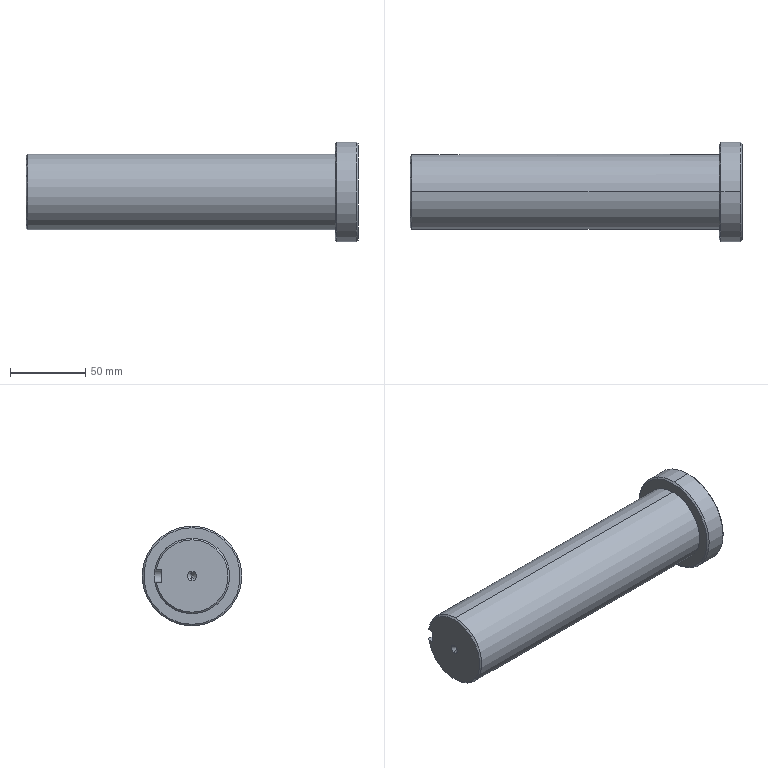Part | SolidWorks | features BaseBody 1 | 1 solid | 22 faces | box 220 x 66 x 66 mm | volume 452201 mm3 | cone 11 | plane 6 | cylinder 5 | commonest cylinder face diameters 50 x2 66 x2 8 x1
STEP:
#1=CARTESIAN_POINT('',(-110.,0.,24.));
#2=VERTEX_POINT('',#1);
#3=CARTESIAN_POINT('',(-110.,23.664,4.));
#4=VERTEX_POINT('',#3);
#5=CARTESIAN_POINT('',(-110.,0.,0.));
#6=DIRECTION('',(-1.,0.,0.));
#7=DIRECTION('',(0.,0.,-1.));
#8=AXIS2_PLACEMENT_3D('',#5,#6,#7);
#9=CIRCLE('',#8,24.);
#10=EDGE_CURVE('',#2,#4,#9,.T.);
#11=ORIENTED_EDGE('',*,*,#10,.F.);
#12=CARTESIAN_POINT('',(-109.,0.,25.));
#13=VERTEX_POINT('',#12);
#14=CARTESIAN_POINT('',(-110.,0.,24.));
#15=DIRECTION('',(0.7071,0.,0.7071));
#16=VECTOR('',#15,1000.);
#17=LINE('',#14,#16);
#18=EDGE_CURVE('',#2,#13,#17,.T.);
#19=ORIENTED_EDGE('',*,*,#18,.T.);
#20=CARTESIAN_POINT('',(-109.,24.678,4.));
#21=VERTEX_POINT('',#20);
#22=CARTESIAN_POINT('',(-109.,0.,0.));
#23=DIRECTION('',(1.,0.,0.));
#24=DIRECTION('',(0.,0.,-1.));
#25=AXIS2_PLACEMENT_3D('',#22,#23,#24);
#26=CIRCLE('',#25,25.);
#27=EDGE_CURVE('',#21,#13,#26,.T.);
#28=ORIENTED_EDGE('',*,*,#27,.F.);
#29=CARTESIAN_POINT('',(-110.,23.664,4.));
#30=CARTESIAN_POINT('',(-109.667,24.002,4.));
#31=CARTESIAN_POINT('',(-109.333,24.34,4.));
#32=CARTESIAN_POINT('',(-109.,24.678,4.));
#33=B_SPLINE_CURVE_WITH_KNOTS('',3,(#29,#30,#31,#32),.UNSPECIFIED.,.F.,.F.,(4,4),(0.007277,0.008701),.UNSPECIFIED.);
#34=EDGE_CURVE('',#4,#21,#33,.T.);
#35=ORIENTED_EDGE('',*,*,#34,.F.);
#36=EDGE_LOOP('',(#11,#19,#28,#35));
#37=FACE_OUTER_BOUND('',#36,.T.);
#38=CARTESIAN_POINT('',(-110.,0.,0.));
#39=DIRECTION('',(1.,0.,0.));
#40=DIRECTION('',(0.,0.,-1.));
#41=AXIS2_PLACEMENT_3D('',#38,#39,#40);
#42=CONICAL_SURFACE('',#41,24.,0.7854);
#43=ADVANCED_FACE('',(#37),#42,.T.);
#44=ORIENTED_EDGE('',*,*,#18,.F.);
#45=CARTESIAN_POINT('',(-110.,0.,-24.));
#46=VERTEX_POINT('',#45);
#47=CARTESIAN_POINT('',(-110.,0.,0.));
#48=DIRECTION('',(-1.,0.,0.));
#49=DIRECTION('',(0.,0.,-1.));
#50=AXIS2_PLACEMENT_3D('',#47,#48,#49);
#51=CIRCLE('',#50,24.);
#52=EDGE_CURVE('',#46,#2,#51,.T.);
#53=ORIENTED_EDGE('',*,*,#52,.F.);
#54=CARTESIAN_POINT('',(-109.,0.,-25.));
#55=VERTEX_POINT('',#54);
#56=CARTESIAN_POINT('',(-110.,0.,-24.));
#57=DIRECTION('',(0.7071,0.,-0.7071));
#58=VECTOR('',#57,1000.);
#59=LINE('',#56,#58);
#60=EDGE_CURVE('',#46,#55,#59,.T.);
#61=ORIENTED_EDGE('',*,*,#60,.T.);
#62=CARTESIAN_POINT('',(-109.,0.,0.));
#63=DIRECTION('',(1.,0.,0.));
#64=DIRECTION('',(0.,0.,-1.));
#65=AXIS2_PLACEMENT_3D('',#62,#63,#64);
#66=CIRCLE('',#65,25.);
#67=EDGE_CURVE('',#13,#55,#66,.T.);
#68=ORIENTED_EDGE('',*,*,#67,.F.);
#69=EDGE_LOOP('',(#44,#53,#61,#68));
#70=FACE_OUTER_BOUND('',#69,.T.);
#71=CARTESIAN_POINT('',(-110.,0.,0.));
#72=DIRECTION('',(1.,0.,0.));
#73=DIRECTION('',(0.,0.,-1.));
#74=AXIS2_PLACEMENT_3D('',#71,#72,#73);
#75=CONICAL_SURFACE('',#74,24.,0.7854);
#76=ADVANCED_FACE('',(#70),#75,.T.);
#77=CARTESIAN_POINT('',(95.,0.,32.));
#78=VERTEX_POINT('',#77);
#79=CARTESIAN_POINT('',(95.,0.,-32.));
#80=VERTEX_POINT('',#79);
#81=CARTESIAN_POINT('',(95.,0.,0.));
#82=DIRECTION('',(-1.,0.,0.));
#83=DIRECTION('',(0.,0.,-1.));
#84=AXIS2_PLACEMENT_3D('',#81,#82,#83);
#85=CIRCLE('',#84,32.);
#86=EDGE_CURVE('',#78,#80,#85,.T.);
#87=ORIENTED_EDGE('',*,*,#86,.F.);
#88=CARTESIAN_POINT('',(96.,0.,33.));
#89=VERTEX_POINT('',#88);
#90=CARTESIAN_POINT('',(95.,0.,32.));
#91=DIRECTION('',(0.7071,0.,0.7071));
#92=VECTOR('',#91,1000.);
#93=LINE('',#90,#92);
#94=EDGE_CURVE('',#78,#89,#93,.T.);
#95=ORIENTED_EDGE('',*,*,#94,.T.);
#96=CARTESIAN_POINT('',(96.,0.,-33.));
#97=VERTEX_POINT('',#96);
#98=CARTESIAN_POINT('',(96.,0.,0.));
#99=DIRECTION('',(1.,0.,0.));
#100=DIRECTION('',(0.,0.,-1.));
#101=AXIS2_PLACEMENT_3D('',#98,#99,#100);
#102=CIRCLE('',#101,33.);
#103=EDGE_CURVE('',#97,#89,#102,.T.);
#104=ORIENTED_EDGE('',*,*,#103,.F.);
#105=CARTESIAN_POINT('',(95.,0.,-32.));
#106=DIRECTION('',(0.7071,0.,-0.7071));
#107=VECTOR('',#106,1000.);
#108=LINE('',#105,#107);
#109=EDGE_CURVE('',#80,#97,#108,.T.);
#110=ORIENTED_EDGE('',*,*,#109,.F.);
#111=EDGE_LOOP('',(#87,#95,#104,#110));
#112=FACE_OUTER_BOUND('',#111,.T.);
#113=CARTESIAN_POINT('',(95.,0.,0.));
#114=DIRECTION('',(1.,0.,0.));
#115=DIRECTION('',(0.,0.,-1.));
#116=AXIS2_PLACEMENT_3D('',#113,#114,#115);
#117=CONICAL_SURFACE('',#116,32.,0.7854);
#118=ADVANCED_FACE('',(#112),#117,.T.);
#119=CARTESIAN_POINT('',(110.,0.,-32.));
#120=VERTEX_POINT('',#119);
#121=CARTESIAN_POINT('',(110.,0.,32.));
#122=VERTEX_POINT('',#121);
#123=CARTESIAN_POINT('',(110.,0.,0.));
#124=DIRECTION('',(1.,0.,0.));
#125=DIRECTION('',(0.,0.,1.));
#126=AXIS2_PLACEMENT_3D('',#123,#124,#125);
#127=CIRCLE('',#126,32.);
#128=EDGE_CURVE('',#120,#122,#127,.T.);
#129=ORIENTED_EDGE('',*,*,#128,.F.);
#130=CARTESIAN_POINT('',(109.,0.,-33.));
#131=VERTEX_POINT('',#130);
#132=CARTESIAN_POINT('',(109.,0.,-33.));
#133=DIRECTION('',(-0.7071,0.,-0.7071));
#134=VECTOR('',#133,1000.);
#135=LINE('',#132,#134);
#136=EDGE_CURVE('',#120,#131,#135,.T.);
#137=ORIENTED_EDGE('',*,*,#136,.T.);
#138=CARTESIAN_POINT('',(109.,0.,33.));
#139=VERTEX_POINT('',#138);
#140=CARTESIAN_POINT('',(109.,0.,0.));
#141=DIRECTION('',(-1.,0.,0.));
#142=DIRECTION('',(0.,0.,1.));
#143=AXIS2_PLACEMENT_3D('',#140,#141,#142);
#144=CIRCLE('',#143,33.);
#145=EDGE_CURVE('',#139,#131,#144,.T.);
#146=ORIENTED_EDGE('',*,*,#145,.F.);
#147=CARTESIAN_POINT('',(109.,0.,33.));
#148=DIRECTION('',(-0.7071,0.,0.7071));
#149=VECTOR('',#148,1000.);
#150=LINE('',#147,#149);
#151=EDGE_CURVE('',#122,#139,#150,.T.);
#152=ORIENTED_EDGE('',*,*,#151,.F.);
#153=EDGE_LOOP('',(#129,#137,#146,#152));
#154=FACE_OUTER_BOUND('',#153,.T.);
#155=CARTESIAN_POINT('',(109.,0.,0.));
#156=DIRECTION('',(-1.,0.,0.));
#157=DIRECTION('',(0.,0.,1.));
#158=AXIS2_PLACEMENT_3D('',#155,#156,#157);
#159=CONICAL_SURFACE('',#158,33.,0.7854);
#160=ADVANCED_FACE('',(#154),#159,.T.);
#161=CARTESIAN_POINT('',(95.,0.,25.));
#162=VERTEX_POINT('',#161);
#163=CARTESIAN_POINT('',(95.,0.,-25.));
#164=VERTEX_POINT('',#163);
#165=CARTESIAN_POINT('',(95.,0.,0.));
#166=DIRECTION('',(-1.,0.,0.));
#167=DIRECTION('',(0.,0.,1.));
#168=AXIS2_PLACEMENT_3D('',#165,#166,#167);
#169=CIRCLE('',#168,25.);
#170=EDGE_CURVE('',#162,#164,#169,.T.);
#171=ORIENTED_EDGE('',*,*,#170,.T.);
#172=CARTESIAN_POINT('',(-107.,0.,-25.));
#173=DIRECTION('',(-1.,0.,0.));
#174=VECTOR('',#173,1000.);
#175=LINE('',#172,#174);
#176=EDGE_CURVE('',#164,#55,#175,.T.);
#177=ORIENTED_EDGE('',*,*,#176,.T.);
#178=CARTESIAN_POINT('',(-109.,24.678,-4.));
#179=VERTEX_POINT('',#178);
#180=CARTESIAN_POINT('',(-109.,0.,0.));
#181=DIRECTION('',(1.,0.,0.));
#182=DIRECTION('',(0.,0.,-1.));
#183=AXIS2_PLACEMENT_3D('',#180,#181,#182);
#184=CIRCLE('',#183,25.);
#185=EDGE_CURVE('',#55,#179,#184,.T.);
#186=ORIENTED_EDGE('',*,*,#185,.T.);
#187=CARTESIAN_POINT('',(-80.,24.678,-4.));
#188=VERTEX_POINT('',#187);
#189=CARTESIAN_POINT('',(-107.,24.678,-4.));
#190=DIRECTION('',(1.,0.,0.));
#191=VECTOR('',#190,1000.);
#192=LINE('',#189,#191);
#193=EDGE_CURVE('',#179,#188,#192,.T.);
#194=ORIENTED_EDGE('',*,*,#193,.T.);
#195=CARTESIAN_POINT('',(-80.,24.678,4.));
#196=VERTEX_POINT('',#195);
#197=CARTESIAN_POINT('',(-80.,24.678,-4.));
#198=CARTESIAN_POINT('',(-79.735,24.678,-4.));
#199=CARTESIAN_POINT('',(-79.475,24.682,-3.974));
#200=CARTESIAN_POINT('',(-78.963,24.698,-3.872));
#201=CARTESIAN_POINT('',(-78.709,24.71,-3.795));
#202=CARTESIAN_POINT('',(-78.225,24.74,-3.594));
#203=CARTESIAN_POINT('',(-77.995,24.758,-3.471));
#204=CARTESIAN_POINT('',(-77.561,24.797,-3.181));
#205=CARTESIAN_POINT('',(-77.356,24.819,-3.013));
#206=CARTESIAN_POINT('',(-76.987,24.86,-2.644));
#207=CARTESIAN_POINT('',(-76.822,24.881,-2.443));
#208=CARTESIAN_POINT('',(-76.53,24.92,-2.006));
#209=CARTESIAN_POINT('',(-76.405,24.938,-1.774));
#210=CARTESIAN_POINT('',(-76.206,24.968,-1.293));
#211=CARTESIAN_POINT('',(-76.129,24.98,-1.041));
#212=CARTESIAN_POINT('',(-76.026,24.996,-0.5241));
#213=CARTESIAN_POINT('',(-76.,25.,-0.2643));
#214=CARTESIAN_POINT('',(-76.,25.,0.2582));
#215=CARTESIAN_POINT('',(-76.026,24.996,0.5237));
#216=CARTESIAN_POINT('',(-76.128,24.98,1.037));
#217=CARTESIAN_POINT('',(-76.203,24.968,1.287));
#218=CARTESIAN_POINT('',(-76.404,24.938,1.771));
#219=CARTESIAN_POINT('',(-76.529,24.92,2.005));
#220=CARTESIAN_POINT('',(-76.818,24.882,2.438));
#221=CARTESIAN_POINT('',(-76.984,24.861,2.64));
#222=CARTESIAN_POINT('',(-77.356,24.818,3.013));
#223=CARTESIAN_POINT('',(-77.558,24.798,3.178));
#224=CARTESIAN_POINT('',(-77.99,24.759,3.468));
#225=CARTESIAN_POINT('',(-78.224,24.741,3.594));
#226=CARTESIAN_POINT('',(-78.708,24.711,3.795));
#227=CARTESIAN_POINT('',(-78.957,24.699,3.87));
#228=CARTESIAN_POINT('',(-79.47,24.682,3.973));
#229=CARTESIAN_POINT('',(-79.735,24.678,4.));
#230=CARTESIAN_POINT('',(-80.,24.678,4.));
#231=B_SPLINE_CURVE_WITH_KNOTS('',3,(#197,#198,#199,#200,#201,#202,#203,#204,#205,#206,#207,#208,#209,#210,#211,#212,#213,#214,#215,#216,#217,#218,#219,#220,#221,#222,#223,#224,#225,#226,#227,#228,#229,#230),.UNSPECIFIED.,.F.,.F.,(4,2,2,2,2,2,2,2,2,2,2,2,2,2,2,2,4),(0.,0.0007827,0.001565,0.002348,0.003131,0.003913,0.004696,0.005479,0.006261,0.007044,0.007827,0.008609,0.009392,0.01017,0.01096,0.01174,0.01252),.UNSPECIFIED.);
#232=EDGE_CURVE('',#188,#196,#231,.T.);
#233=ORIENTED_EDGE('',*,*,#232,.T.);
#234=CARTESIAN_POINT('',(-107.,24.678,4.));
#235=DIRECTION('',(-1.,0.,0.));
#236=VECTOR('',#235,1000.);
#237=LINE('',#234,#236);
#238=EDGE_CURVE('',#196,#21,#237,.T.);
#239=ORIENTED_EDGE('',*,*,#238,.T.);
#240=ORIENTED_EDGE('',*,*,#27,.T.);
#241=CARTESIAN_POINT('',(-107.,0.,25.));
#242=DIRECTION('',(-1.,0.,0.));
#243=VECTOR('',#242,1000.);
#244=LINE('',#241,#243);
#245=EDGE_CURVE('',#162,#13,#244,.T.);
#246=ORIENTED_EDGE('',*,*,#245,.F.);
#247=EDGE_LOOP('',(#171,#177,#186,#194,#233,#239,#240,#246));
#248=FACE_OUTER_BOUND('',#247,.T.);
#249=CARTESIAN_POINT('',(-107.,0.,0.));
#250=DIRECTION('',(-1.,0.,0.));
#251=DIRECTION('',(0.,0.,1.));
#252=AXIS2_PLACEMENT_3D('',#249,#250,#251);
#253=CYLINDRICAL_SURFACE('',#252,25.);
#254=ADVANCED_FACE('',(#248),#253,.T.);
#255=ORIENTED_EDGE('',*,*,#145,.T.);
#256=CARTESIAN_POINT('',(-107.,0.,-33.));
#257=DIRECTION('',(-1.,0.,0.));
#258=VECTOR('',#257,1000.);
#259=LINE('',#256,#258);
#260=EDGE_CURVE('',#131,#97,#259,.T.);
#261=ORIENTED_EDGE('',*,*,#260,.T.);
#262=ORIENTED_EDGE('',*,*,#103,.T.);
#263=CARTESIAN_POINT('',(-107.,0.,33.));
#264=DIRECTION('',(-1.,0.,0.));
#265=VECTOR('',#264,1000.);
#266=LINE('',#263,#265);
#267=EDGE_CURVE('',#139,#89,#266,.T.);
#268=ORIENTED_EDGE('',*,*,#267,.F.);
#269=EDGE_LOOP('',(#255,#261,#262,#268));
#270=FACE_OUTER_BOUND('',#269,.T.);
#271=CARTESIAN_POINT('',(-107.,0.,0.));
#272=DIRECTION('',(-1.,0.,0.));
#273=DIRECTION('',(0.,0.,1.));
#274=AXIS2_PLACEMENT_3D('',#271,#272,#273);
#275=CYLINDRICAL_SURFACE('',#274,33.);
#276=ADVANCED_FACE('',(#270),#275,.T.);
#277=CARTESIAN_POINT('',(107.,0.,0.));
#278=VERTEX_POINT('',#277);
#279=CARTESIAN_POINT('',(110.,0.,-3.));
#280=VERTEX_POINT('',#279);
#281=CARTESIAN_POINT('',(107.,0.,0.));
#282=DIRECTION('',(0.7071,0.,-0.7071));
#283=VECTOR('',#282,1000.);
#284=LINE('',#281,#283);
#285=EDGE_CURVE('',#278,#280,#284,.T.);
#286=ORIENTED_EDGE('',*,*,#285,.F.);
#287=CARTESIAN_POINT('',(110.,0.,3.));
#288=VERTEX_POINT('',#287);
#289=CARTESIAN_POINT('',(107.,0.,0.));
#290=DIRECTION('',(0.7071,0.,0.7071));
#291=VECTOR('',#290,1000.);
#292=LINE('',#289,#291);
#293=EDGE_CURVE('',#278,#288,#292,.T.);
#294=ORIENTED_EDGE('',*,*,#293,.T.);
#295=CARTESIAN_POINT('',(110.,0.,0.));
#296=DIRECTION('',(-1.,0.,0.));
#297=DIRECTION('',(0.,0.,1.));
#298=AXIS2_PLACEMENT_3D('',#295,#296,#297);
#299=CIRCLE('',#298,3.);
#300=EDGE_CURVE('',#280,#288,#299,.T.);
#301=ORIENTED_EDGE('',*,*,#300,.F.);
#302=EDGE_LOOP('',(#286,#294,#301));
#303=FACE_OUTER_BOUND('',#302,.T.);
#304=CARTESIAN_POINT('',(1107.,0.,0.));
#305=DIRECTION('',(1.,0.,0.));
#306=DIRECTION('',(0.,0.,-1.));
#307=AXIS2_PLACEMENT_3D('',#304,#305,#306);
#308=CONICAL_SURFACE('',#307,1000.,0.7854);
#309=ADVANCED_FACE('',(#303),#308,.F.);
#310=CARTESIAN_POINT('',(-107.,0.,0.));
#311=VERTEX_POINT('',#310);
#312=CARTESIAN_POINT('',(-110.,0.,3.));
#313=VERTEX_POINT('',#312);
#314=CARTESIAN_POINT('',(-110.,0.,3.));
#315=DIRECTION('',(-0.7071,0.,0.7071));
#316=VECTOR('',#315,1000.);
#317=LINE('',#314,#316);
#318=EDGE_CURVE('',#311,#313,#317,.T.);
#319=ORIENTED_EDGE('',*,*,#318,.F.);
#320=CARTESIAN_POINT('',(-110.,0.,-3.));
#321=VERTEX_POINT('',#320);
#322=CARTESIAN_POINT('',(-110.,0.,-3.));
#323=DIRECTION('',(-0.7071,0.,-0.7071));
#324=VECTOR('',#323,1000.);
#325=LINE('',#322,#324);
#326=EDGE_CURVE('',#311,#321,#325,.T.);
#327=ORIENTED_EDGE('',*,*,#326,.T.);
#328=CARTESIAN_POINT('',(-110.,0.,0.));
#329=DIRECTION('',(-1.,0.,0.));
#330=DIRECTION('',(0.,0.,1.));
#331=AXIS2_PLACEMENT_3D('',#328,#329,#330);
#332=CIRCLE('',#331,3.);
#333=EDGE_CURVE('',#321,#313,#332,.T.);
#334=ORIENTED_EDGE('',*,*,#333,.T.);
#335=EDGE_LOOP('',(#319,#327,#334));
#336=FACE_OUTER_BOUND('',#335,.T.);
#337=CARTESIAN_POINT('',(-110.,0.,0.));
#338=DIRECTION('',(-1.,0.,0.));
#339=DIRECTION('',(0.,0.,1.));
#340=AXIS2_PLACEMENT_3D('',#337,#338,#339);
#341=CONICAL_SURFACE('',#340,3.,0.7854);
#342=ADVANCED_FACE('',(#336),#341,.F.);
#343=ORIENTED_EDGE('',*,*,#326,.F.);
#344=ORIENTED_EDGE('',*,*,#318,.T.);
#345=CARTESIAN_POINT('',(-110.,0.,0.));
#346=DIRECTION('',(-1.,0.,0.));
#347=DIRECTION('',(0.,0.,1.));
#348=AXIS2_PLACEMENT_3D('',#345,#346,#347);
#349=CIRCLE('',#348,3.);
#350=EDGE_CURVE('',#313,#321,#349,.T.);
#351=ORIENTED_EDGE('',*,*,#350,.T.);
#352=EDGE_LOOP('',(#343,#344,#351));
#353=FACE_OUTER_BOUND('',#352,.T.);
#354=CARTESIAN_POINT('',(-110.,0.,0.));
#355=DIRECTION('',(-1.,0.,0.));
#356=DIRECTION('',(0.,0.,1.));
#357=AXIS2_PLACEMENT_3D('',#354,#355,#356);
#358=CONICAL_SURFACE('',#357,3.,0.7854);
#359=ADVANCED_FACE('',(#353),#358,.F.);
#360=ORIENTED_EDGE('',*,*,#293,.F.);
#361=ORIENTED_EDGE('',*,*,#285,.T.);
#362=CARTESIAN_POINT('',(110.,0.,0.));
#363=DIRECTION('',(-1.,0.,0.));
#364=DIRECTION('',(0.,0.,1.));
#365=AXIS2_PLACEMENT_3D('',#362,#363,#364);
#366=CIRCLE('',#365,3.);
#367=EDGE_CURVE('',#288,#280,#366,.T.);
#368=ORIENTED_EDGE('',*,*,#367,.F.);
#369=EDGE_LOOP('',(#360,#361,#368));
#370=FACE_OUTER_BOUND('',#369,.T.);
#371=CARTESIAN_POINT('',(1107.,0.,0.));
#372=DIRECTION('',(1.,0.,0.));
#373=DIRECTION('',(0.,0.,-1.));
#374=AXIS2_PLACEMENT_3D('',#371,#372,#373);
#375=CONICAL_SURFACE('',#374,1000.,0.7854);
#376=ADVANCED_FACE('',(#370),#375,.F.);
#377=CARTESIAN_POINT('',(110.,0.,0.));
#378=DIRECTION('',(1.,0.,0.));
#379=DIRECTION('',(0.,0.,1.));
#380=AXIS2_PLACEMENT_3D('',#377,#378,#379);
#381=CIRCLE('',#380,32.);
#382=EDGE_CURVE('',#122,#120,#381,.T.);
#383=ORIENTED_EDGE('',*,*,#382,.T.);
#384=ORIENTED_EDGE('',*,*,#128,.T.);
#385=EDGE_LOOP('',(#383,#384));
#386=FACE_OUTER_BOUND('',#385,.T.);
#387=ORIENTED_EDGE('',*,*,#300,.T.);
#388=ORIENTED_EDGE('',*,*,#367,.T.);
#389=EDGE_LOOP('',(#387,#388));
#390=FACE_BOUND('',#389,.T.);
#391=CARTESIAN_POINT('',(110.,0.,-3.));
#392=DIRECTION('',(-1.,0.,0.));
#393=DIRECTION('',(0.,0.,1.));
#394=AXIS2_PLACEMENT_3D('',#391,#392,#393);
#395=PLANE('',#394);
#396=ADVANCED_FACE('',(#386,#390),#395,.F.);
#397=ORIENTED_EDGE('',*,*,#260,.F.);
#398=CARTESIAN_POINT('',(109.,0.,0.));
#399=DIRECTION('',(-1.,0.,0.));
#400=DIRECTION('',(0.,0.,1.));
#401=AXIS2_PLACEMENT_3D('',#398,#399,#400);
#402=CIRCLE('',#401,33.);
#403=EDGE_CURVE('',#131,#139,#402,.T.);
#404=ORIENTED_EDGE('',*,*,#403,.T.);
#405=ORIENTED_EDGE('',*,*,#267,.T.);
#406=CARTESIAN_POINT('',(96.,0.,0.));
#407=DIRECTION('',(1.,0.,0.));
#408=DIRECTION('',(0.,0.,-1.));
#409=AXIS2_PLACEMENT_3D('',#406,#407,#408);
#410=CIRCLE('',#409,33.);
#411=EDGE_CURVE('',#89,#97,#410,.T.);
#412=ORIENTED_EDGE('',*,*,#411,.T.);
#413=EDGE_LOOP('',(#397,#404,#405,#412));
#414=FACE_OUTER_BOUND('',#413,.T.);
#415=CARTESIAN_POINT('',(-107.,0.,0.));
#416=DIRECTION('',(-1.,0.,0.));
#417=DIRECTION('',(0.,0.,1.));
#418=AXIS2_PLACEMENT_3D('',#415,#416,#417);
#419=CYLINDRICAL_SURFACE('',#418,33.);
#420=ADVANCED_FACE('',(#414),#419,.T.);
#421=CARTESIAN_POINT('',(95.,0.,0.));
#422=DIRECTION('',(-1.,0.,0.));
#423=DIRECTION('',(0.,0.,-1.));
#424=AXIS2_PLACEMENT_3D('',#421,#422,#423);
#425=CIRCLE('',#424,32.);
#426=EDGE_CURVE('',#80,#78,#425,.T.);
#427=ORIENTED_EDGE('',*,*,#426,.T.);
#428=ORIENTED_EDGE('',*,*,#86,.T.);
#429=EDGE_LOOP('',(#427,#428));
#430=FACE_OUTER_BOUND('',#429,.T.);
#431=ORIENTED_EDGE('',*,*,#170,.F.);
#432=CARTESIAN_POINT('',(95.,0.,0.));
#433=DIRECTION('',(-1.,0.,0.));
#434=DIRECTION('',(0.,0.,1.));
#435=AXIS2_PLACEMENT_3D('',#432,#433,#434);
#436=CIRCLE('',#435,25.);
#437=EDGE_CURVE('',#164,#162,#436,.T.);
#438=ORIENTED_EDGE('',*,*,#437,.F.);
#439=EDGE_LOOP('',(#431,#438));
#440=FACE_BOUND('',#439,.T.);
#441=CARTESIAN_POINT('',(95.,0.,-33.));
#442=DIRECTION('',(1.,0.,0.));
#443=DIRECTION('',(0.,0.,-1.));
#444=AXIS2_PLACEMENT_3D('',#441,#442,#443);
#445=PLANE('',#444);
#446=ADVANCED_FACE('',(#430,#440),#445,.F.);
#447=ORIENTED_EDGE('',*,*,#176,.F.);
#448=ORIENTED_EDGE('',*,*,#437,.T.);
#449=ORIENTED_EDGE('',*,*,#245,.T.);
#450=ORIENTED_EDGE('',*,*,#67,.T.);
#451=EDGE_LOOP('',(#447,#448,#449,#450));
#452=FACE_OUTER_BOUND('',#451,.T.);
#453=CARTESIAN_POINT('',(-107.,0.,0.));
#454=DIRECTION('',(-1.,0.,0.));
#455=DIRECTION('',(0.,0.,1.));
#456=AXIS2_PLACEMENT_3D('',#453,#454,#455);
#457=CYLINDRICAL_SURFACE('',#456,25.);
#458=ADVANCED_FACE('',(#452),#457,.T.);
#459=CARTESIAN_POINT('',(-110.,20.,-4.));
#460=VERTEX_POINT('',#459);
#461=CARTESIAN_POINT('',(-110.,20.,4.));
#462=VERTEX_POINT('',#461);
#463=CARTESIAN_POINT('',(-110.,20.,-25.));
#464=DIRECTION('',(0.,0.,1.));
#465=VECTOR('',#464,1000.);
#466=LINE('',#463,#465);
#467=EDGE_CURVE('',#460,#462,#466,.T.);
#468=ORIENTED_EDGE('',*,*,#467,.F.);
#469=CARTESIAN_POINT('',(-110.,23.664,-4.));
#470=VERTEX_POINT('',#469);
#471=CARTESIAN_POINT('',(-110.,20.,-4.));
#472=DIRECTION('',(0.,1.,0.));
#473=VECTOR('',#472,1000.);
#474=LINE('',#471,#473);
#475=EDGE_CURVE('',#460,#470,#474,.T.);
#476=ORIENTED_EDGE('',*,*,#475,.T.);
#477=CARTESIAN_POINT('',(-110.,0.,0.));
#478=DIRECTION('',(-1.,0.,0.));
#479=DIRECTION('',(0.,0.,-1.));
#480=AXIS2_PLACEMENT_3D('',#477,#478,#479);
#481=CIRCLE('',#480,24.);
#482=EDGE_CURVE('',#470,#46,#481,.T.);
#483=ORIENTED_EDGE('',*,*,#482,.T.);
#484=ORIENTED_EDGE('',*,*,#52,.T.);
#485=ORIENTED_EDGE('',*,*,#10,.T.);
#486=CARTESIAN_POINT('',(-110.,20.,4.));
#487=DIRECTION('',(0.,1.,0.));
#488=VECTOR('',#487,1000.);
#489=LINE('',#486,#488);
#490=EDGE_CURVE('',#462,#4,#489,.T.);
#491=ORIENTED_EDGE('',*,*,#490,.F.);
#492=EDGE_LOOP('',(#468,#476,#483,#484,#485,#491));
#493=FACE_OUTER_BOUND('',#492,.T.);
#494=ORIENTED_EDGE('',*,*,#350,.F.);
#495=ORIENTED_EDGE('',*,*,#333,.F.);
#496=EDGE_LOOP('',(#494,#495));
#497=FACE_BOUND('',#496,.T.);
#498=CARTESIAN_POINT('',(-110.,0.,-25.));
#499=DIRECTION('',(1.,0.,0.));
#500=DIRECTION('',(0.,0.,-1.));
#501=AXIS2_PLACEMENT_3D('',#498,#499,#500);
#502=PLANE('',#501);
#503=ADVANCED_FACE('',(#493,#497),#502,.F.);
#504=ORIENTED_EDGE('',*,*,#136,.F.);
#505=ORIENTED_EDGE('',*,*,#382,.F.);
#506=ORIENTED_EDGE('',*,*,#151,.T.);
#507=ORIENTED_EDGE('',*,*,#403,.F.);
#508=EDGE_LOOP('',(#504,#505,#506,#507));
#509=FACE_OUTER_BOUND('',#508,.T.);
#510=CARTESIAN_POINT('',(109.,0.,0.));
#511=DIRECTION('',(-1.,0.,0.));
#512=DIRECTION('',(0.,0.,1.));
#513=AXIS2_PLACEMENT_3D('',#510,#511,#512);
#514=CONICAL_SURFACE('',#513,33.,0.7854);
#515=ADVANCED_FACE('',(#509),#514,.T.);
#516=ORIENTED_EDGE('',*,*,#94,.F.);
#517=ORIENTED_EDGE('',*,*,#426,.F.);
#518=ORIENTED_EDGE('',*,*,#109,.T.);
#519=ORIENTED_EDGE('',*,*,#411,.F.);
#520=EDGE_LOOP('',(#516,#517,#518,#519));
#521=FACE_OUTER_BOUND('',#520,.T.);
#522=CARTESIAN_POINT('',(95.,0.,0.));
#523=DIRECTION('',(1.,0.,0.));
#524=DIRECTION('',(0.,0.,-1.));
#525=AXIS2_PLACEMENT_3D('',#522,#523,#524);
#526=CONICAL_SURFACE('',#525,32.,0.7854);
#527=ADVANCED_FACE('',(#521),#526,.T.);
#528=ORIENTED_EDGE('',*,*,#60,.F.);
#529=ORIENTED_EDGE('',*,*,#482,.F.);
#530=CARTESIAN_POINT('',(-109.,24.678,-4.));
#531=CARTESIAN_POINT('',(-109.333,24.34,-4.));
#532=CARTESIAN_POINT('',(-109.667,24.002,-4.));
#533=CARTESIAN_POINT('',(-110.,23.664,-4.));
#534=B_SPLINE_CURVE_WITH_KNOTS('',3,(#530,#531,#532,#533),.UNSPECIFIED.,.F.,.F.,(4,4),(0.00725,0.008674),.UNSPECIFIED.);
#535=EDGE_CURVE('',#179,#470,#534,.T.);
#536=ORIENTED_EDGE('',*,*,#535,.F.);
#537=ORIENTED_EDGE('',*,*,#185,.F.);
#538=EDGE_LOOP('',(#528,#529,#536,#537));
#539=FACE_OUTER_BOUND('',#538,.T.);
#540=CARTESIAN_POINT('',(-110.,0.,0.));
#541=DIRECTION('',(1.,0.,0.));
#542=DIRECTION('',(0.,0.,-1.));
#543=AXIS2_PLACEMENT_3D('',#540,#541,#542);
#544=CONICAL_SURFACE('',#543,24.,0.7854);
#545=ADVANCED_FACE('',(#539),#544,.T.);
#546=CARTESIAN_POINT('',(-80.,20.,-4.));
#547=VERTEX_POINT('',#546);
#548=CARTESIAN_POINT('',(-80.,20.,-4.));
#549=DIRECTION('',(0.,1.,0.));
#550=VECTOR('',#549,1000.);
#551=LINE('',#548,#550);
#552=EDGE_CURVE('',#547,#188,#551,.T.);
#553=ORIENTED_EDGE('',*,*,#552,.F.);
#554=CARTESIAN_POINT('',(-80.,20.,4.));
#555=VERTEX_POINT('',#554);
#556=CARTESIAN_POINT('',(-80.,20.,0.));
#557=DIRECTION('',(0.,1.,0.));
#558=DIRECTION('',(0.,0.,1.));
#559=AXIS2_PLACEMENT_3D('',#556,#557,#558);
#560=CIRCLE('',#559,4.);
#561=EDGE_CURVE('',#555,#547,#560,.T.);
#562=ORIENTED_EDGE('',*,*,#561,.F.);
#563=CARTESIAN_POINT('',(-80.,20.,4.));
#564=DIRECTION('',(0.,1.,0.));
#565=VECTOR('',#564,1000.);
#566=LINE('',#563,#565);
#567=EDGE_CURVE('',#555,#196,#566,.T.);
#568=ORIENTED_EDGE('',*,*,#567,.T.);
#569=ORIENTED_EDGE('',*,*,#232,.F.);
#570=EDGE_LOOP('',(#553,#562,#568,#569));
#571=FACE_OUTER_BOUND('',#570,.T.);
#572=CARTESIAN_POINT('',(-80.,20.,0.));
#573=DIRECTION('',(0.,1.,0.));
#574=DIRECTION('',(0.,0.,1.));
#575=AXIS2_PLACEMENT_3D('',#572,#573,#574);
#576=CYLINDRICAL_SURFACE('',#575,4.);
#577=ADVANCED_FACE('',(#571),#576,.F.);
#578=ORIENTED_EDGE('',*,*,#467,.T.);
#579=CARTESIAN_POINT('',(-110.,20.,4.));
#580=DIRECTION('',(1.,0.,0.));
#581=VECTOR('',#580,1000.);
#582=LINE('',#579,#581);
#583=EDGE_CURVE('',#462,#555,#582,.T.);
#584=ORIENTED_EDGE('',*,*,#583,.T.);
#585=ORIENTED_EDGE('',*,*,#561,.T.);
#586=CARTESIAN_POINT('',(-110.,20.,-4.));
#587=DIRECTION('',(-1.,0.,0.));
#588=VECTOR('',#587,1000.);
#589=LINE('',#586,#588);
#590=EDGE_CURVE('',#547,#460,#589,.T.);
#591=ORIENTED_EDGE('',*,*,#590,.T.);
#592=EDGE_LOOP('',(#578,#584,#585,#591));
#593=FACE_OUTER_BOUND('',#592,.T.);
#594=CARTESIAN_POINT('',(-110.,20.,0.));
#595=DIRECTION('',(0.,1.,0.));
#596=DIRECTION('',(0.,0.,1.));
#597=AXIS2_PLACEMENT_3D('',#594,#595,#596);
#598=PLANE('',#597);
#599=ADVANCED_FACE('',(#593),#598,.T.);
#600=ORIENTED_EDGE('',*,*,#535,.T.);
#601=ORIENTED_EDGE('',*,*,#475,.F.);
#602=ORIENTED_EDGE('',*,*,#590,.F.);
#603=ORIENTED_EDGE('',*,*,#552,.T.);
#604=ORIENTED_EDGE('',*,*,#193,.F.);
#605=EDGE_LOOP('',(#600,#601,#602,#603,#604));
#606=FACE_OUTER_BOUND('',#605,.T.);
#607=CARTESIAN_POINT('',(-110.,20.,-4.));
#608=DIRECTION('',(0.,0.,-1.));
#609=DIRECTION('',(-1.,0.,0.));
#610=AXIS2_PLACEMENT_3D('',#607,#608,#609);
#611=PLANE('',#610);
#612=ADVANCED_FACE('',(#606),#611,.F.);
#613=ORIENTED_EDGE('',*,*,#567,.F.);
#614=ORIENTED_EDGE('',*,*,#583,.F.);
#615=ORIENTED_EDGE('',*,*,#490,.T.);
#616=ORIENTED_EDGE('',*,*,#34,.T.);
#617=ORIENTED_EDGE('',*,*,#238,.F.);
#618=EDGE_LOOP('',(#613,#614,#615,#616,#617));
#619=FACE_OUTER_BOUND('',#618,.T.);
#620=CARTESIAN_POINT('',(-110.,20.,4.));
#621=DIRECTION('',(0.,0.,1.));
#622=DIRECTION('',(1.,0.,0.));
#623=AXIS2_PLACEMENT_3D('',#620,#621,#622);
#624=PLANE('',#623);
#625=ADVANCED_FACE('',(#619),#624,.F.);
#626=CLOSED_SHELL('',(#43,#76,#118,#160,#254,#276,#309,#342,#359,#376,#396,#420,#446,#458,#503,#515,#527,#545,#577,#599,#612,#625));
#627=MANIFOLD_SOLID_BREP('',#626);
#628=CARTESIAN_POINT('',(0.,0.,0.));
#629=DIRECTION('',(0.,0.,1.));
#630=DIRECTION('',(1.,0.,0.));
#631=AXIS2_PLACEMENT_3D('',#628,#629,#630);
#632=(LENGTH_UNIT()NAMED_UNIT(*)SI_UNIT(.MILLI.,.METRE.));
#633=UNCERTAINTY_MEASURE_WITH_UNIT(LENGTH_MEASURE(0.00001),#632,'','');
#634=(NAMED_UNIT(*)PLANE_ANGLE_UNIT()SI_UNIT($,.RADIAN.));
#635=(NAMED_UNIT(*)SI_UNIT($,.STERADIAN.)SOLID_ANGLE_UNIT());
#636=(GEOMETRIC_REPRESENTATION_CONTEXT(3)GLOBAL_UNCERTAINTY_ASSIGNED_CONTEXT((#633))GLOBAL_UNIT_ASSIGNED_CONTEXT((#632,#634,#635))REPRESENTATION_CONTEXT('',''));
#637=ADVANCED_BREP_SHAPE_REPRESENTATION('',(#627,#631),#636);